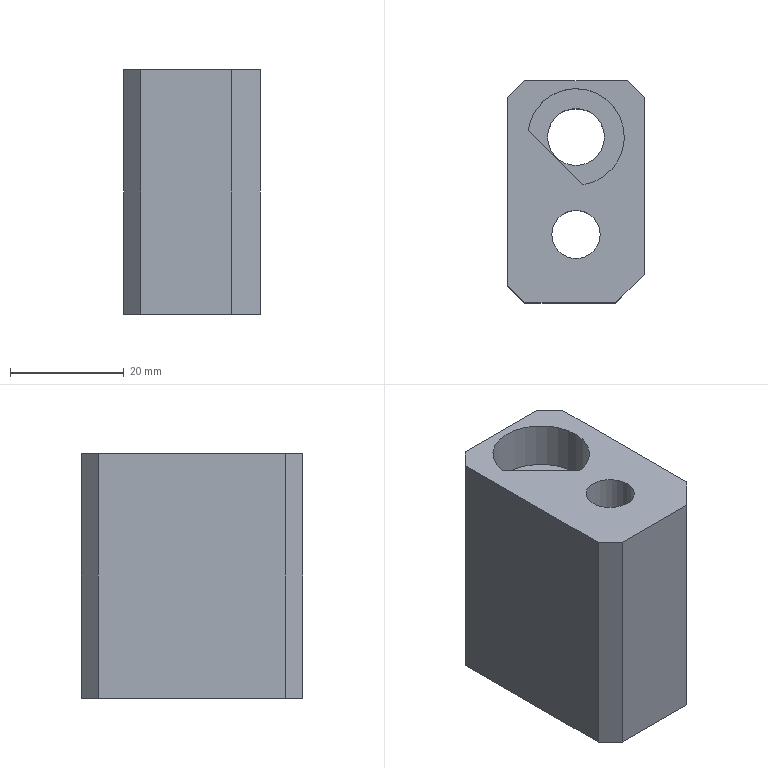Part | NX | features PH-4 2 | 1 solid | 17 faces | box 24 x 39 x 43 mm | volume 31156 mm3 | plane 13 | cylinder 4 | commonest cylinder face diameters 8.5 x1 10.001 x1 14.5 x1 17 x1
STEP:
#1=CARTESIAN_POINT('',(2393.285,-796.145,945.716));
#2=VERTEX_POINT('',#1);
#3=CARTESIAN_POINT('',(2402.901,-805.762,945.716));
#4=VERTEX_POINT('',#3);
#5=CARTESIAN_POINT('',(2398.093,-800.953,945.716));
#6=DIRECTION('',(0.7071,-0.7071,0.));
#7=VECTOR('',#6,1000.);
#8=LINE('',#5,#7);
#9=EDGE_CURVE('',#2,#4,#8,.T.);
#10=ORIENTED_EDGE('',*,*,#9,.F.);
#11=CARTESIAN_POINT('',(2401.699,-797.347,945.716));
#12=DIRECTION('',(0.,0.,-1.));
#13=DIRECTION('',(1.,0.,0.));
#14=AXIS2_PLACEMENT_3D('',#11,#12,#13);
#15=CIRCLE('',#14,8.5);
#16=EDGE_CURVE('',#2,#4,#15,.T.);
#17=ORIENTED_EDGE('',*,*,#16,.T.);
#18=EDGE_LOOP('',(#10,#17));
#19=FACE_BOUND('',#18,.T.);
#20=CARTESIAN_POINT('',(2405.949,-814.497,945.716));
#21=VERTEX_POINT('',#20);
#22=CARTESIAN_POINT('',(2401.699,-814.497,945.716));
#23=DIRECTION('',(0.,0.,1.));
#24=DIRECTION('',(1.,0.,0.));
#25=AXIS2_PLACEMENT_3D('',#22,#23,#24);
#26=CIRCLE('',#25,4.25);
#27=EDGE_CURVE('',#21,#21,#26,.T.);
#28=ORIENTED_EDGE('',*,*,#27,.F.);
#29=EDGE_LOOP('',(#28));
#30=FACE_BOUND('',#29,.T.);
#31=CARTESIAN_POINT('',(2408.699,-826.497,945.716));
#32=VERTEX_POINT('',#31);
#33=CARTESIAN_POINT('',(2392.699,-826.497,945.716));
#34=VERTEX_POINT('',#33);
#35=CARTESIAN_POINT('',(2401.699,-826.497,945.716));
#36=DIRECTION('',(-1.,0.,0.));
#37=VECTOR('',#36,1000.);
#38=LINE('',#35,#37);
#39=EDGE_CURVE('',#32,#34,#38,.T.);
#40=ORIENTED_EDGE('',*,*,#39,.F.);
#41=CARTESIAN_POINT('',(2413.699,-821.497,945.716));
#42=VERTEX_POINT('',#41);
#43=CARTESIAN_POINT('',(2414.949,-820.247,945.716));
#44=DIRECTION('',(-0.7071,-0.7071,0.));
#45=VECTOR('',#44,1000.);
#46=LINE('',#43,#45);
#47=EDGE_CURVE('',#32,#42,#46,.F.);
#48=ORIENTED_EDGE('',*,*,#47,.T.);
#49=CARTESIAN_POINT('',(2413.699,-790.497,945.716));
#50=VERTEX_POINT('',#49);
#51=CARTESIAN_POINT('',(2413.699,-806.997,945.716));
#52=DIRECTION('',(0.,-1.,0.));
#53=VECTOR('',#52,1000.);
#54=LINE('',#51,#53);
#55=EDGE_CURVE('',#50,#42,#54,.T.);
#56=ORIENTED_EDGE('',*,*,#55,.F.);
#57=CARTESIAN_POINT('',(2410.699,-787.497,945.716));
#58=VERTEX_POINT('',#57);
#59=CARTESIAN_POINT('',(2415.949,-792.747,945.716));
#60=DIRECTION('',(0.7071,-0.7071,0.));
#61=VECTOR('',#60,1000.);
#62=LINE('',#59,#61);
#63=EDGE_CURVE('',#50,#58,#62,.F.);
#64=ORIENTED_EDGE('',*,*,#63,.T.);
#65=CARTESIAN_POINT('',(2392.699,-787.497,945.716));
#66=VERTEX_POINT('',#65);
#67=CARTESIAN_POINT('',(2401.699,-787.497,945.716));
#68=DIRECTION('',(1.,0.,0.));
#69=VECTOR('',#68,1000.);
#70=LINE('',#67,#69);
#71=EDGE_CURVE('',#66,#58,#70,.T.);
#72=ORIENTED_EDGE('',*,*,#71,.F.);
#73=CARTESIAN_POINT('',(2389.699,-790.497,945.716));
#74=VERTEX_POINT('',#73);
#75=CARTESIAN_POINT('',(2387.449,-792.747,945.716));
#76=DIRECTION('',(0.7071,0.7071,0.));
#77=VECTOR('',#76,1000.);
#78=LINE('',#75,#77);
#79=EDGE_CURVE('',#66,#74,#78,.F.);
#80=ORIENTED_EDGE('',*,*,#79,.T.);
#81=CARTESIAN_POINT('',(2389.699,-823.497,945.716));
#82=VERTEX_POINT('',#81);
#83=CARTESIAN_POINT('',(2389.699,-806.997,945.716));
#84=DIRECTION('',(0.,1.,0.));
#85=VECTOR('',#84,1000.);
#86=LINE('',#83,#85);
#87=EDGE_CURVE('',#82,#74,#86,.T.);
#88=ORIENTED_EDGE('',*,*,#87,.F.);
#89=CARTESIAN_POINT('',(2387.449,-821.247,945.716));
#90=DIRECTION('',(-0.7071,0.7071,0.));
#91=VECTOR('',#90,1000.);
#92=LINE('',#89,#91);
#93=EDGE_CURVE('',#82,#34,#92,.F.);
#94=ORIENTED_EDGE('',*,*,#93,.T.);
#95=EDGE_LOOP('',(#40,#48,#56,#64,#72,#80,#88,#94));
#96=FACE_BOUND('',#95,.T.);
#97=CARTESIAN_POINT('',(2401.699,-806.997,945.716));
#98=DIRECTION('',(0.,0.,1.));
#99=DIRECTION('',(-1.,0.,0.));
#100=AXIS2_PLACEMENT_3D('',#97,#98,#99);
#101=PLANE('',#100);
#102=ADVANCED_FACE('',(#19,#30,#96),#101,.T.);
#103=CARTESIAN_POINT('',(2410.699,-787.497,902.716));
#104=VERTEX_POINT('',#103);
#105=CARTESIAN_POINT('',(2392.699,-787.497,902.716));
#106=VERTEX_POINT('',#105);
#107=CARTESIAN_POINT('',(2401.699,-787.497,902.716));
#108=DIRECTION('',(-1.,0.,0.));
#109=VECTOR('',#108,1000.);
#110=LINE('',#107,#109);
#111=EDGE_CURVE('',#104,#106,#110,.T.);
#112=ORIENTED_EDGE('',*,*,#111,.T.);
#113=CARTESIAN_POINT('',(2392.699,-787.497,920.716));
#114=DIRECTION('',(0.,0.,1.));
#115=VECTOR('',#114,1000.);
#116=LINE('',#113,#115);
#117=EDGE_CURVE('',#106,#66,#116,.T.);
#118=ORIENTED_EDGE('',*,*,#117,.T.);
#119=ORIENTED_EDGE('',*,*,#71,.T.);
#120=CARTESIAN_POINT('',(2410.699,-787.497,920.716));
#121=DIRECTION('',(0.,0.,-1.));
#122=VECTOR('',#121,1000.);
#123=LINE('',#120,#122);
#124=EDGE_CURVE('',#58,#104,#123,.T.);
#125=ORIENTED_EDGE('',*,*,#124,.T.);
#126=EDGE_LOOP('',(#112,#118,#119,#125));
#127=FACE_BOUND('',#126,.T.);
#128=CARTESIAN_POINT('',(2401.699,-787.497,920.716));
#129=DIRECTION('',(0.,1.,0.));
#130=DIRECTION('',(0.,0.,-1.));
#131=AXIS2_PLACEMENT_3D('',#128,#129,#130);
#132=PLANE('',#131);
#133=ADVANCED_FACE('',(#127),#132,.T.);
#134=ORIENTED_EDGE('',*,*,#55,.T.);
#135=CARTESIAN_POINT('',(2413.699,-821.497,902.716));
#136=VERTEX_POINT('',#135);
#137=CARTESIAN_POINT('',(2413.699,-821.497,920.716));
#138=DIRECTION('',(0.,0.,-1.));
#139=VECTOR('',#138,1000.);
#140=LINE('',#137,#139);
#141=EDGE_CURVE('',#42,#136,#140,.T.);
#142=ORIENTED_EDGE('',*,*,#141,.T.);
#143=CARTESIAN_POINT('',(2413.699,-790.497,902.716));
#144=VERTEX_POINT('',#143);
#145=CARTESIAN_POINT('',(2413.699,-806.997,902.716));
#146=DIRECTION('',(0.,1.,0.));
#147=VECTOR('',#146,1000.);
#148=LINE('',#145,#147);
#149=EDGE_CURVE('',#136,#144,#148,.T.);
#150=ORIENTED_EDGE('',*,*,#149,.T.);
#151=CARTESIAN_POINT('',(2413.699,-790.497,920.716));
#152=DIRECTION('',(0.,0.,1.));
#153=VECTOR('',#152,1000.);
#154=LINE('',#151,#153);
#155=EDGE_CURVE('',#144,#50,#154,.T.);
#156=ORIENTED_EDGE('',*,*,#155,.T.);
#157=EDGE_LOOP('',(#134,#142,#150,#156));
#158=FACE_BOUND('',#157,.T.);
#159=CARTESIAN_POINT('',(2413.699,-806.997,920.716));
#160=DIRECTION('',(1.,0.,0.));
#161=DIRECTION('',(0.,0.,1.));
#162=AXIS2_PLACEMENT_3D('',#159,#160,#161);
#163=PLANE('',#162);
#164=ADVANCED_FACE('',(#158),#163,.T.);
#165=CARTESIAN_POINT('',(2392.699,-826.497,902.716));
#166=VERTEX_POINT('',#165);
#167=CARTESIAN_POINT('',(2408.699,-826.497,902.716));
#168=VERTEX_POINT('',#167);
#169=CARTESIAN_POINT('',(2401.699,-826.497,902.716));
#170=DIRECTION('',(1.,0.,0.));
#171=VECTOR('',#170,1000.);
#172=LINE('',#169,#171);
#173=EDGE_CURVE('',#166,#168,#172,.T.);
#174=ORIENTED_EDGE('',*,*,#173,.T.);
#175=CARTESIAN_POINT('',(2408.699,-826.497,920.716));
#176=DIRECTION('',(0.,0.,1.));
#177=VECTOR('',#176,1000.);
#178=LINE('',#175,#177);
#179=EDGE_CURVE('',#168,#32,#178,.T.);
#180=ORIENTED_EDGE('',*,*,#179,.T.);
#181=ORIENTED_EDGE('',*,*,#39,.T.);
#182=CARTESIAN_POINT('',(2392.699,-826.497,920.716));
#183=DIRECTION('',(0.,0.,-1.));
#184=VECTOR('',#183,1000.);
#185=LINE('',#182,#184);
#186=EDGE_CURVE('',#34,#166,#185,.T.);
#187=ORIENTED_EDGE('',*,*,#186,.T.);
#188=EDGE_LOOP('',(#174,#180,#181,#187));
#189=FACE_BOUND('',#188,.T.);
#190=CARTESIAN_POINT('',(2401.699,-826.497,920.716));
#191=DIRECTION('',(0.,-1.,0.));
#192=DIRECTION('',(0.,0.,1.));
#193=AXIS2_PLACEMENT_3D('',#190,#191,#192);
#194=PLANE('',#193);
#195=ADVANCED_FACE('',(#189),#194,.T.);
#196=CARTESIAN_POINT('',(2396.699,-797.347,902.716));
#197=VERTEX_POINT('',#196);
#198=CARTESIAN_POINT('',(2401.699,-797.347,902.716));
#199=DIRECTION('',(0.,0.,-1.));
#200=DIRECTION('',(-1.,0.,0.));
#201=AXIS2_PLACEMENT_3D('',#198,#199,#200);
#202=CIRCLE('',#201,5.);
#203=EDGE_CURVE('',#197,#197,#202,.T.);
#204=ORIENTED_EDGE('',*,*,#203,.F.);
#205=EDGE_LOOP('',(#204));
#206=FACE_BOUND('',#205,.T.);
#207=CARTESIAN_POINT('',(2394.449,-814.497,902.716));
#208=VERTEX_POINT('',#207);
#209=CARTESIAN_POINT('',(2401.699,-814.497,902.716));
#210=DIRECTION('',(0.,0.,-1.));
#211=DIRECTION('',(-1.,0.,0.));
#212=AXIS2_PLACEMENT_3D('',#209,#210,#211);
#213=CIRCLE('',#212,7.25);
#214=EDGE_CURVE('',#208,#208,#213,.F.);
#215=ORIENTED_EDGE('',*,*,#214,.T.);
#216=EDGE_LOOP('',(#215));
#217=FACE_BOUND('',#216,.T.);
#218=ORIENTED_EDGE('',*,*,#149,.F.);
#219=CARTESIAN_POINT('',(2414.949,-820.247,902.716));
#220=DIRECTION('',(0.7071,0.7071,0.));
#221=VECTOR('',#220,1000.);
#222=LINE('',#219,#221);
#223=EDGE_CURVE('',#136,#168,#222,.F.);
#224=ORIENTED_EDGE('',*,*,#223,.T.);
#225=ORIENTED_EDGE('',*,*,#173,.F.);
#226=CARTESIAN_POINT('',(2389.699,-823.497,902.716));
#227=VERTEX_POINT('',#226);
#228=CARTESIAN_POINT('',(2387.449,-821.247,902.716));
#229=DIRECTION('',(0.7071,-0.7071,0.));
#230=VECTOR('',#229,1000.);
#231=LINE('',#228,#230);
#232=EDGE_CURVE('',#166,#227,#231,.F.);
#233=ORIENTED_EDGE('',*,*,#232,.T.);
#234=CARTESIAN_POINT('',(2389.699,-790.497,902.716));
#235=VERTEX_POINT('',#234);
#236=CARTESIAN_POINT('',(2389.699,-806.997,902.716));
#237=DIRECTION('',(0.,-1.,0.));
#238=VECTOR('',#237,1000.);
#239=LINE('',#236,#238);
#240=EDGE_CURVE('',#235,#227,#239,.T.);
#241=ORIENTED_EDGE('',*,*,#240,.F.);
#242=CARTESIAN_POINT('',(2387.449,-792.747,902.716));
#243=DIRECTION('',(-0.7071,-0.7071,0.));
#244=VECTOR('',#243,1000.);
#245=LINE('',#242,#244);
#246=EDGE_CURVE('',#235,#106,#245,.F.);
#247=ORIENTED_EDGE('',*,*,#246,.T.);
#248=ORIENTED_EDGE('',*,*,#111,.F.);
#249=CARTESIAN_POINT('',(2415.949,-792.747,902.716));
#250=DIRECTION('',(-0.7071,0.7071,0.));
#251=VECTOR('',#250,1000.);
#252=LINE('',#249,#251);
#253=EDGE_CURVE('',#104,#144,#252,.F.);
#254=ORIENTED_EDGE('',*,*,#253,.T.);
#255=EDGE_LOOP('',(#218,#224,#225,#233,#241,#247,#248,#254));
#256=FACE_BOUND('',#255,.T.);
#257=CARTESIAN_POINT('',(2401.699,-806.997,902.716));
#258=DIRECTION('',(0.,0.,-1.));
#259=DIRECTION('',(1.,0.,0.));
#260=AXIS2_PLACEMENT_3D('',#257,#258,#259);
#261=PLANE('',#260);
#262=ADVANCED_FACE('',(#206,#217,#256),#261,.T.);
#263=ORIENTED_EDGE('',*,*,#240,.T.);
#264=CARTESIAN_POINT('',(2389.699,-823.497,920.716));
#265=DIRECTION('',(0.,0.,1.));
#266=VECTOR('',#265,1000.);
#267=LINE('',#264,#266);
#268=EDGE_CURVE('',#227,#82,#267,.T.);
#269=ORIENTED_EDGE('',*,*,#268,.T.);
#270=ORIENTED_EDGE('',*,*,#87,.T.);
#271=CARTESIAN_POINT('',(2389.699,-790.497,920.716));
#272=DIRECTION('',(0.,0.,-1.));
#273=VECTOR('',#272,1000.);
#274=LINE('',#271,#273);
#275=EDGE_CURVE('',#74,#235,#274,.T.);
#276=ORIENTED_EDGE('',*,*,#275,.T.);
#277=EDGE_LOOP('',(#263,#269,#270,#276));
#278=FACE_BOUND('',#277,.T.);
#279=CARTESIAN_POINT('',(2389.699,-806.997,920.716));
#280=DIRECTION('',(-1.,0.,0.));
#281=DIRECTION('',(0.,0.,-1.));
#282=AXIS2_PLACEMENT_3D('',#279,#280,#281);
#283=PLANE('',#282);
#284=ADVANCED_FACE('',(#278),#283,.T.);
#285=ORIENTED_EDGE('',*,*,#232,.F.);
#286=ORIENTED_EDGE('',*,*,#186,.F.);
#287=ORIENTED_EDGE('',*,*,#93,.F.);
#288=ORIENTED_EDGE('',*,*,#268,.F.);
#289=EDGE_LOOP('',(#285,#286,#287,#288));
#290=FACE_BOUND('',#289,.T.);
#291=CARTESIAN_POINT('',(2389.699,-823.497,920.716));
#292=DIRECTION('',(0.7071,0.7071,0.));
#293=DIRECTION('',(-0.7071,0.7071,0.));
#294=AXIS2_PLACEMENT_3D('',#291,#292,#293);
#295=PLANE('',#294);
#296=ADVANCED_FACE('',(#290),#295,.F.);
#297=ORIENTED_EDGE('',*,*,#246,.F.);
#298=ORIENTED_EDGE('',*,*,#275,.F.);
#299=ORIENTED_EDGE('',*,*,#79,.F.);
#300=ORIENTED_EDGE('',*,*,#117,.F.);
#301=EDGE_LOOP('',(#297,#298,#299,#300));
#302=FACE_BOUND('',#301,.T.);
#303=CARTESIAN_POINT('',(2392.699,-787.497,920.716));
#304=DIRECTION('',(0.7071,-0.7071,0.));
#305=DIRECTION('',(0.7071,0.7071,0.));
#306=AXIS2_PLACEMENT_3D('',#303,#304,#305);
#307=PLANE('',#306);
#308=ADVANCED_FACE('',(#302),#307,.F.);
#309=ORIENTED_EDGE('',*,*,#253,.F.);
#310=ORIENTED_EDGE('',*,*,#124,.F.);
#311=ORIENTED_EDGE('',*,*,#63,.F.);
#312=ORIENTED_EDGE('',*,*,#155,.F.);
#313=EDGE_LOOP('',(#309,#310,#311,#312));
#314=FACE_BOUND('',#313,.T.);
#315=CARTESIAN_POINT('',(2413.699,-790.497,920.716));
#316=DIRECTION('',(-0.7071,-0.7071,0.));
#317=DIRECTION('',(0.7071,-0.7071,0.));
#318=AXIS2_PLACEMENT_3D('',#315,#316,#317);
#319=PLANE('',#318);
#320=ADVANCED_FACE('',(#314),#319,.F.);
#321=CARTESIAN_POINT('',(2405.949,-814.497,913.716));
#322=VERTEX_POINT('',#321);
#323=CARTESIAN_POINT('',(2401.699,-814.497,913.716));
#324=DIRECTION('',(0.,0.,1.));
#325=DIRECTION('',(1.,0.,0.));
#326=AXIS2_PLACEMENT_3D('',#323,#324,#325);
#327=CIRCLE('',#326,4.25);
#328=EDGE_CURVE('',#322,#322,#327,.T.);
#329=ORIENTED_EDGE('',*,*,#328,.T.);
#330=EDGE_LOOP('',(#329));
#331=FACE_BOUND('',#330,.T.);
#332=CARTESIAN_POINT('',(2408.949,-814.497,913.716));
#333=VERTEX_POINT('',#332);
#334=CARTESIAN_POINT('',(2401.699,-814.497,913.716));
#335=DIRECTION('',(0.,0.,1.));
#336=DIRECTION('',(1.,0.,0.));
#337=AXIS2_PLACEMENT_3D('',#334,#335,#336);
#338=CIRCLE('',#337,7.25);
#339=EDGE_CURVE('',#333,#333,#338,.T.);
#340=ORIENTED_EDGE('',*,*,#339,.F.);
#341=EDGE_LOOP('',(#340));
#342=FACE_BOUND('',#341,.T.);
#343=CARTESIAN_POINT('',(2401.699,-814.497,913.716));
#344=DIRECTION('',(0.,0.,1.));
#345=DIRECTION('',(1.,0.,0.));
#346=AXIS2_PLACEMENT_3D('',#343,#344,#345);
#347=PLANE('',#346);
#348=ADVANCED_FACE('',(#331,#342),#347,.F.);
#349=ORIENTED_EDGE('',*,*,#214,.F.);
#350=EDGE_LOOP('',(#349));
#351=FACE_BOUND('',#350,.T.);
#352=ORIENTED_EDGE('',*,*,#339,.T.);
#353=EDGE_LOOP('',(#352));
#354=FACE_BOUND('',#353,.T.);
#355=CARTESIAN_POINT('',(2401.699,-814.497,931.716));
#356=DIRECTION('',(0.,0.,-1.));
#357=DIRECTION('',(-1.,0.,0.));
#358=AXIS2_PLACEMENT_3D('',#355,#356,#357);
#359=CYLINDRICAL_SURFACE('',#358,7.25);
#360=ADVANCED_FACE('',(#351,#354),#359,.F.);
#361=ORIENTED_EDGE('',*,*,#27,.T.);
#362=EDGE_LOOP('',(#361));
#363=FACE_BOUND('',#362,.T.);
#364=ORIENTED_EDGE('',*,*,#328,.F.);
#365=EDGE_LOOP('',(#364));
#366=FACE_BOUND('',#365,.T.);
#367=CARTESIAN_POINT('',(2401.699,-814.497,946.716));
#368=DIRECTION('',(0.,0.,-1.));
#369=DIRECTION('',(-1.,0.,0.));
#370=AXIS2_PLACEMENT_3D('',#367,#368,#369);
#371=CYLINDRICAL_SURFACE('',#370,4.25);
#372=ADVANCED_FACE('',(#363,#366),#371,.F.);
#373=CARTESIAN_POINT('',(2402.901,-805.762,937.416));
#374=VERTEX_POINT('',#373);
#375=CARTESIAN_POINT('',(2393.285,-796.145,937.416));
#376=VERTEX_POINT('',#375);
#377=CARTESIAN_POINT('',(2398.093,-800.953,937.416));
#378=DIRECTION('',(-0.7071,0.7071,0.));
#379=VECTOR('',#378,1000.);
#380=LINE('',#377,#379);
#381=EDGE_CURVE('',#374,#376,#380,.T.);
#382=ORIENTED_EDGE('',*,*,#381,.F.);
#383=CARTESIAN_POINT('',(2401.699,-797.347,937.416));
#384=DIRECTION('',(0.,0.,1.));
#385=DIRECTION('',(1.,0.,0.));
#386=AXIS2_PLACEMENT_3D('',#383,#384,#385);
#387=CIRCLE('',#386,8.5);
#388=EDGE_CURVE('',#374,#376,#387,.T.);
#389=ORIENTED_EDGE('',*,*,#388,.T.);
#390=EDGE_LOOP('',(#382,#389));
#391=FACE_BOUND('',#390,.T.);
#392=CARTESIAN_POINT('',(2396.699,-797.347,937.416));
#393=VERTEX_POINT('',#392);
#394=CARTESIAN_POINT('',(2401.699,-797.347,937.416));
#395=DIRECTION('',(0.,0.,-1.));
#396=DIRECTION('',(-1.,0.,0.));
#397=AXIS2_PLACEMENT_3D('',#394,#395,#396);
#398=CIRCLE('',#397,5.);
#399=EDGE_CURVE('',#393,#393,#398,.F.);
#400=ORIENTED_EDGE('',*,*,#399,.F.);
#401=EDGE_LOOP('',(#400));
#402=FACE_BOUND('',#401,.T.);
#403=CARTESIAN_POINT('',(2401.699,-797.347,937.416));
#404=DIRECTION('',(0.,0.,-1.));
#405=DIRECTION('',(-1.,0.,0.));
#406=AXIS2_PLACEMENT_3D('',#403,#404,#405);
#407=PLANE('',#406);
#408=ADVANCED_FACE('',(#391,#402),#407,.F.);
#409=ORIENTED_EDGE('',*,*,#47,.F.);
#410=ORIENTED_EDGE('',*,*,#179,.F.);
#411=ORIENTED_EDGE('',*,*,#223,.F.);
#412=ORIENTED_EDGE('',*,*,#141,.F.);
#413=EDGE_LOOP('',(#409,#410,#411,#412));
#414=FACE_BOUND('',#413,.T.);
#415=CARTESIAN_POINT('',(2413.699,-821.497,920.716));
#416=DIRECTION('',(-0.7071,0.7071,0.));
#417=DIRECTION('',(0.,0.,-1.));
#418=AXIS2_PLACEMENT_3D('',#415,#416,#417);
#419=PLANE('',#418);
#420=ADVANCED_FACE('',(#414),#419,.F.);
#421=ORIENTED_EDGE('',*,*,#9,.T.);
#422=CARTESIAN_POINT('',(2402.901,-805.762,945.716));
#423=DIRECTION('',(0.,0.,-1.));
#424=VECTOR('',#423,1000.);
#425=LINE('',#422,#424);
#426=EDGE_CURVE('',#374,#4,#425,.F.);
#427=ORIENTED_EDGE('',*,*,#426,.F.);
#428=ORIENTED_EDGE('',*,*,#381,.T.);
#429=CARTESIAN_POINT('',(2393.285,-796.145,945.716));
#430=DIRECTION('',(0.,0.,-1.));
#431=VECTOR('',#430,1000.);
#432=LINE('',#429,#431);
#433=EDGE_CURVE('',#2,#376,#432,.T.);
#434=ORIENTED_EDGE('',*,*,#433,.F.);
#435=EDGE_LOOP('',(#421,#427,#428,#434));
#436=FACE_BOUND('',#435,.T.);
#437=CARTESIAN_POINT('',(2398.093,-800.953,960.966));
#438=DIRECTION('',(-0.7071,-0.7071,0.));
#439=DIRECTION('',(0.7071,-0.7071,0.));
#440=AXIS2_PLACEMENT_3D('',#437,#438,#439);
#441=PLANE('',#440);
#442=ADVANCED_FACE('',(#436),#441,.F.);
#443=ORIENTED_EDGE('',*,*,#388,.F.);
#444=ORIENTED_EDGE('',*,*,#426,.T.);
#445=ORIENTED_EDGE('',*,*,#16,.F.);
#446=ORIENTED_EDGE('',*,*,#433,.T.);
#447=EDGE_LOOP('',(#443,#444,#445,#446));
#448=FACE_BOUND('',#447,.T.);
#449=CARTESIAN_POINT('',(2401.699,-797.347,945.716));
#450=DIRECTION('',(0.,0.,-1.));
#451=DIRECTION('',(1.,0.,0.));
#452=AXIS2_PLACEMENT_3D('',#449,#450,#451);
#453=CYLINDRICAL_SURFACE('',#452,8.5);
#454=ADVANCED_FACE('',(#448),#453,.F.);
#455=ORIENTED_EDGE('',*,*,#203,.T.);
#456=EDGE_LOOP('',(#455));
#457=FACE_BOUND('',#456,.T.);
#458=ORIENTED_EDGE('',*,*,#399,.T.);
#459=EDGE_LOOP('',(#458));
#460=FACE_BOUND('',#459,.T.);
#461=CARTESIAN_POINT('',(2401.699,-797.347,945.716));
#462=DIRECTION('',(0.,0.,-1.));
#463=DIRECTION('',(1.,0.,0.));
#464=AXIS2_PLACEMENT_3D('',#461,#462,#463);
#465=CYLINDRICAL_SURFACE('',#464,5.);
#466=ADVANCED_FACE('',(#457,#460),#465,.F.);
#467=CLOSED_SHELL('',(#102,#133,#164,#195,#262,#284,#296,#308,#320,#348,#360,#372,#408,#420,#442,#454,#466));
#468=MANIFOLD_SOLID_BREP('',#467);
#469=(LENGTH_UNIT()NAMED_UNIT(*)SI_UNIT(.MILLI.,.METRE.));
#470=UNCERTAINTY_MEASURE_WITH_UNIT(LENGTH_MEASURE(0.00001),#469,'','');
#471=(NAMED_UNIT(*)PLANE_ANGLE_UNIT()SI_UNIT($,.RADIAN.));
#472=(NAMED_UNIT(*)SI_UNIT($,.STERADIAN.)SOLID_ANGLE_UNIT());
#473=(GEOMETRIC_REPRESENTATION_CONTEXT(3)GLOBAL_UNCERTAINTY_ASSIGNED_CONTEXT((#470))GLOBAL_UNIT_ASSIGNED_CONTEXT((#469,#471,#472))REPRESENTATION_CONTEXT('',''));
#474=ADVANCED_BREP_SHAPE_REPRESENTATION('',(#468),#473);